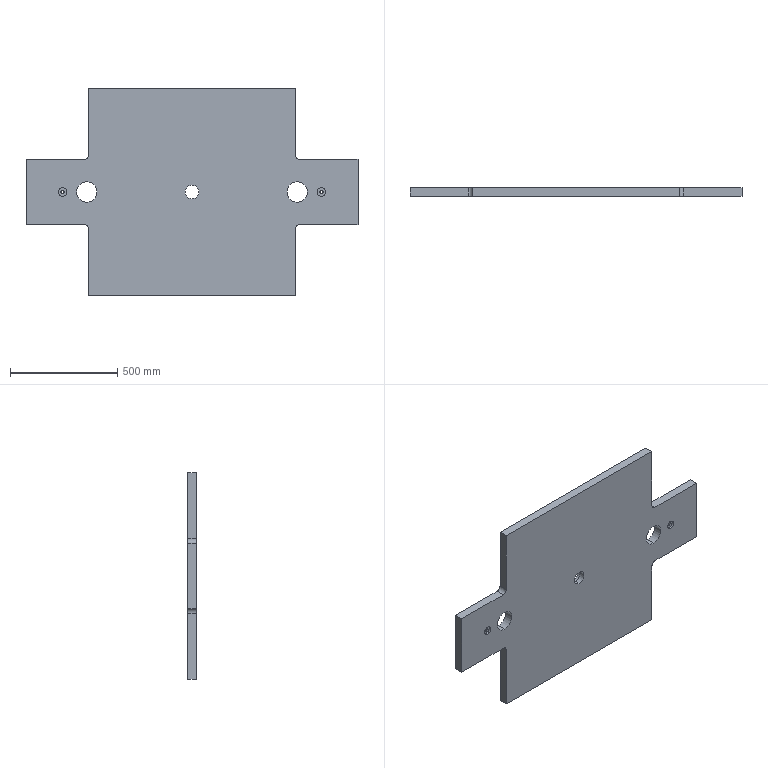Part | SolidWorks | features Cut 4, MirrorPattern 2, Extrusion 1, Fillet 1, HoleWzd 1 | 1 solid | 43 faces | box 1546 x 40 x 960 mm | volume 43281864 mm3 | cylinder 24 | plane 19 | commonest cylinder face diameters 40 x8 15.5 x4 24 x4 95 x4 63.5 x2 68 x2
STEP:
#1=CARTESIAN_POINT('',(0.,25.,-34.));
#2=VERTEX_POINT('',#1);
#3=CARTESIAN_POINT('',(0.,25.,34.));
#4=VERTEX_POINT('',#3);
#5=CARTESIAN_POINT('',(0.,25.,0.));
#6=DIRECTION('',(0.,1.,0.));
#7=DIRECTION('',(0.,0.,1.));
#8=AXIS2_PLACEMENT_3D('',#5,#6,#7);
#9=CIRCLE('',#8,34.);
#10=EDGE_CURVE('',#2,#4,#9,.T.);
#11=ORIENTED_EDGE('',*,*,#10,.F.);
#12=CARTESIAN_POINT('',(0.,40.,-34.));
#13=VERTEX_POINT('',#12);
#14=CARTESIAN_POINT('',(0.,25.,-34.));
#15=DIRECTION('',(0.,1.,0.));
#16=VECTOR('',#15,1000.);
#17=LINE('',#14,#16);
#18=EDGE_CURVE('',#2,#13,#17,.T.);
#19=ORIENTED_EDGE('',*,*,#18,.T.);
#20=CARTESIAN_POINT('',(0.,40.,34.));
#21=VERTEX_POINT('',#20);
#22=CARTESIAN_POINT('',(0.,40.,0.));
#23=DIRECTION('',(0.,1.,0.));
#24=DIRECTION('',(0.,0.,1.));
#25=AXIS2_PLACEMENT_3D('',#22,#23,#24);
#26=CIRCLE('',#25,34.);
#27=EDGE_CURVE('',#13,#21,#26,.T.);
#28=ORIENTED_EDGE('',*,*,#27,.T.);
#29=CARTESIAN_POINT('',(0.,25.,34.));
#30=DIRECTION('',(0.,1.,0.));
#31=VECTOR('',#30,1000.);
#32=LINE('',#29,#31);
#33=EDGE_CURVE('',#4,#21,#32,.T.);
#34=ORIENTED_EDGE('',*,*,#33,.F.);
#35=EDGE_LOOP('',(#11,#19,#28,#34));
#36=FACE_OUTER_BOUND('',#35,.T.);
#37=CARTESIAN_POINT('',(0.,25.,0.));
#38=DIRECTION('',(0.,1.,0.));
#39=DIRECTION('',(0.,0.,1.));
#40=AXIS2_PLACEMENT_3D('',#37,#38,#39);
#41=CYLINDRICAL_SURFACE('',#40,34.);
#42=ADVANCED_FACE('',(#36),#41,.F.);
#43=CARTESIAN_POINT('',(-490.,40.,-47.5));
#44=VERTEX_POINT('',#43);
#45=CARTESIAN_POINT('',(-490.,40.,47.5));
#46=VERTEX_POINT('',#45);
#47=CARTESIAN_POINT('',(-490.,40.,0.));
#48=DIRECTION('',(0.,1.,0.));
#49=DIRECTION('',(0.,0.,-1.));
#50=AXIS2_PLACEMENT_3D('',#47,#48,#49);
#51=CIRCLE('',#50,47.5);
#52=EDGE_CURVE('',#44,#46,#51,.T.);
#53=ORIENTED_EDGE('',*,*,#52,.T.);
#54=CARTESIAN_POINT('',(-490.,0.,47.5));
#55=VERTEX_POINT('',#54);
#56=CARTESIAN_POINT('',(-490.,40.,47.5));
#57=DIRECTION('',(0.,-1.,0.));
#58=VECTOR('',#57,1000.);
#59=LINE('',#56,#58);
#60=EDGE_CURVE('',#46,#55,#59,.T.);
#61=ORIENTED_EDGE('',*,*,#60,.T.);
#62=CARTESIAN_POINT('',(-490.,0.,-47.5));
#63=VERTEX_POINT('',#62);
#64=CARTESIAN_POINT('',(-490.,0.,0.));
#65=DIRECTION('',(0.,1.,0.));
#66=DIRECTION('',(0.,0.,-1.));
#67=AXIS2_PLACEMENT_3D('',#64,#65,#66);
#68=CIRCLE('',#67,47.5);
#69=EDGE_CURVE('',#63,#55,#68,.T.);
#70=ORIENTED_EDGE('',*,*,#69,.F.);
#71=CARTESIAN_POINT('',(-490.,40.,-47.5));
#72=DIRECTION('',(0.,-1.,0.));
#73=VECTOR('',#72,1000.);
#74=LINE('',#71,#73);
#75=EDGE_CURVE('',#44,#63,#74,.T.);
#76=ORIENTED_EDGE('',*,*,#75,.F.);
#77=EDGE_LOOP('',(#53,#61,#70,#76));
#78=FACE_OUTER_BOUND('',#77,.T.);
#79=CARTESIAN_POINT('',(-490.,40.,0.));
#80=DIRECTION('',(0.,-1.,0.));
#81=DIRECTION('',(0.,0.,-1.));
#82=AXIS2_PLACEMENT_3D('',#79,#80,#81);
#83=CYLINDRICAL_SURFACE('',#82,47.5);
#84=ADVANCED_FACE('',(#78),#83,.F.);
#85=CARTESIAN_POINT('',(490.,40.,47.5));
#86=VERTEX_POINT('',#85);
#87=CARTESIAN_POINT('',(490.,40.,-47.5));
#88=VERTEX_POINT('',#87);
#89=CARTESIAN_POINT('',(490.,40.,0.));
#90=DIRECTION('',(0.,-1.,0.));
#91=DIRECTION('',(0.,0.,-1.));
#92=AXIS2_PLACEMENT_3D('',#89,#90,#91);
#93=CIRCLE('',#92,47.5);
#94=EDGE_CURVE('',#86,#88,#93,.T.);
#95=ORIENTED_EDGE('',*,*,#94,.F.);
#96=CARTESIAN_POINT('',(490.,0.,47.5));
#97=VERTEX_POINT('',#96);
#98=CARTESIAN_POINT('',(490.,40.,47.5));
#99=DIRECTION('',(0.,-1.,0.));
#100=VECTOR('',#99,1000.);
#101=LINE('',#98,#100);
#102=EDGE_CURVE('',#86,#97,#101,.T.);
#103=ORIENTED_EDGE('',*,*,#102,.T.);
#104=CARTESIAN_POINT('',(490.,0.,-47.5));
#105=VERTEX_POINT('',#104);
#106=CARTESIAN_POINT('',(490.,0.,0.));
#107=DIRECTION('',(0.,-1.,0.));
#108=DIRECTION('',(0.,0.,-1.));
#109=AXIS2_PLACEMENT_3D('',#106,#107,#108);
#110=CIRCLE('',#109,47.5);
#111=EDGE_CURVE('',#97,#105,#110,.T.);
#112=ORIENTED_EDGE('',*,*,#111,.T.);
#113=CARTESIAN_POINT('',(490.,40.,-47.5));
#114=DIRECTION('',(0.,-1.,0.));
#115=VECTOR('',#114,1000.);
#116=LINE('',#113,#115);
#117=EDGE_CURVE('',#88,#105,#116,.T.);
#118=ORIENTED_EDGE('',*,*,#117,.F.);
#119=EDGE_LOOP('',(#95,#103,#112,#118));
#120=FACE_OUTER_BOUND('',#119,.T.);
#121=CARTESIAN_POINT('',(490.,40.,0.));
#122=DIRECTION('',(0.,-1.,0.));
#123=DIRECTION('',(0.,0.,-1.));
#124=AXIS2_PLACEMENT_3D('',#121,#122,#123);
#125=CYLINDRICAL_SURFACE('',#124,47.5);
#126=ADVANCED_FACE('',(#120),#125,.F.);
#127=CARTESIAN_POINT('',(-602.5,25.,-12.));
#128=VERTEX_POINT('',#127);
#129=CARTESIAN_POINT('',(-602.5,25.,12.));
#130=VERTEX_POINT('',#129);
#131=CARTESIAN_POINT('',(-602.5,25.,0.));
#132=DIRECTION('',(0.,1.,0.));
#133=DIRECTION('',(0.,0.,1.));
#134=AXIS2_PLACEMENT_3D('',#131,#132,#133);
#135=CIRCLE('',#134,12.);
#136=EDGE_CURVE('',#128,#130,#135,.T.);
#137=ORIENTED_EDGE('',*,*,#136,.F.);
#138=CARTESIAN_POINT('',(-602.5,40.,-12.));
#139=VERTEX_POINT('',#138);
#140=CARTESIAN_POINT('',(-602.5,40.,-12.));
#141=DIRECTION('',(0.,1.,0.));
#142=VECTOR('',#141,1000.);
#143=LINE('',#140,#142);
#144=EDGE_CURVE('',#128,#139,#143,.T.);
#145=ORIENTED_EDGE('',*,*,#144,.T.);
#146=CARTESIAN_POINT('',(-602.5,40.,12.));
#147=VERTEX_POINT('',#146);
#148=CARTESIAN_POINT('',(-602.5,40.,0.));
#149=DIRECTION('',(0.,1.,0.));
#150=DIRECTION('',(0.,0.,1.));
#151=AXIS2_PLACEMENT_3D('',#148,#149,#150);
#152=CIRCLE('',#151,12.);
#153=EDGE_CURVE('',#139,#147,#152,.T.);
#154=ORIENTED_EDGE('',*,*,#153,.T.);
#155=CARTESIAN_POINT('',(-602.5,40.,12.));
#156=DIRECTION('',(0.,1.,0.));
#157=VECTOR('',#156,1000.);
#158=LINE('',#155,#157);
#159=EDGE_CURVE('',#130,#147,#158,.T.);
#160=ORIENTED_EDGE('',*,*,#159,.F.);
#161=EDGE_LOOP('',(#137,#145,#154,#160));
#162=FACE_OUTER_BOUND('',#161,.T.);
#163=CARTESIAN_POINT('',(-602.5,40.,0.));
#164=DIRECTION('',(0.,1.,0.));
#165=DIRECTION('',(0.,0.,1.));
#166=AXIS2_PLACEMENT_3D('',#163,#164,#165);
#167=CYLINDRICAL_SURFACE('',#166,12.);
#168=ADVANCED_FACE('',(#162),#167,.F.);
#169=CARTESIAN_POINT('',(-602.5,10.,7.75));
#170=VERTEX_POINT('',#169);
#171=CARTESIAN_POINT('',(-602.5,10.,-7.75));
#172=VERTEX_POINT('',#171);
#173=CARTESIAN_POINT('',(-602.5,10.,0.));
#174=DIRECTION('',(0.,-1.,0.));
#175=DIRECTION('',(0.,0.,-1.));
#176=AXIS2_PLACEMENT_3D('',#173,#174,#175);
#177=CIRCLE('',#176,7.75);
#178=EDGE_CURVE('',#170,#172,#177,.T.);
#179=ORIENTED_EDGE('',*,*,#178,.T.);
#180=CARTESIAN_POINT('',(-602.5,25.,-7.75));
#181=VERTEX_POINT('',#180);
#182=CARTESIAN_POINT('',(-602.5,40.,-7.75));
#183=DIRECTION('',(0.,1.,0.));
#184=VECTOR('',#183,1000.);
#185=LINE('',#182,#184);
#186=EDGE_CURVE('',#172,#181,#185,.T.);
#187=ORIENTED_EDGE('',*,*,#186,.T.);
#188=CARTESIAN_POINT('',(-602.5,25.,7.75));
#189=VERTEX_POINT('',#188);
#190=CARTESIAN_POINT('',(-602.5,25.,0.));
#191=DIRECTION('',(0.,1.,0.));
#192=DIRECTION('',(0.,0.,1.));
#193=AXIS2_PLACEMENT_3D('',#190,#191,#192);
#194=CIRCLE('',#193,7.75);
#195=EDGE_CURVE('',#181,#189,#194,.T.);
#196=ORIENTED_EDGE('',*,*,#195,.T.);
#197=CARTESIAN_POINT('',(-602.5,40.,7.75));
#198=DIRECTION('',(0.,1.,0.));
#199=VECTOR('',#198,1000.);
#200=LINE('',#197,#199);
#201=EDGE_CURVE('',#170,#189,#200,.T.);
#202=ORIENTED_EDGE('',*,*,#201,.F.);
#203=EDGE_LOOP('',(#179,#187,#196,#202));
#204=FACE_OUTER_BOUND('',#203,.T.);
#205=CARTESIAN_POINT('',(-602.5,40.,0.));
#206=DIRECTION('',(0.,1.,0.));
#207=DIRECTION('',(0.,0.,1.));
#208=AXIS2_PLACEMENT_3D('',#205,#206,#207);
#209=CYLINDRICAL_SURFACE('',#208,7.75);
#210=ADVANCED_FACE('',(#204),#209,.F.);
#211=CARTESIAN_POINT('',(-602.5,10.,-20.));
#212=VERTEX_POINT('',#211);
#213=CARTESIAN_POINT('',(-602.5,10.,20.));
#214=VERTEX_POINT('',#213);
#215=CARTESIAN_POINT('',(-602.5,10.,0.));
#216=DIRECTION('',(0.,1.,0.));
#217=DIRECTION('',(0.,0.,-1.));
#218=AXIS2_PLACEMENT_3D('',#215,#216,#217);
#219=CIRCLE('',#218,20.);
#220=EDGE_CURVE('',#212,#214,#219,.T.);
#221=ORIENTED_EDGE('',*,*,#220,.T.);
#222=CARTESIAN_POINT('',(-602.5,0.,20.));
#223=VERTEX_POINT('',#222);
#224=CARTESIAN_POINT('',(-602.5,10.,20.));
#225=DIRECTION('',(0.,-1.,0.));
#226=VECTOR('',#225,1000.);
#227=LINE('',#224,#226);
#228=EDGE_CURVE('',#214,#223,#227,.T.);
#229=ORIENTED_EDGE('',*,*,#228,.T.);
#230=CARTESIAN_POINT('',(-602.5,0.,-20.));
#231=VERTEX_POINT('',#230);
#232=CARTESIAN_POINT('',(-602.5,0.,0.));
#233=DIRECTION('',(0.,1.,0.));
#234=DIRECTION('',(0.,0.,-1.));
#235=AXIS2_PLACEMENT_3D('',#232,#233,#234);
#236=CIRCLE('',#235,20.);
#237=EDGE_CURVE('',#231,#223,#236,.T.);
#238=ORIENTED_EDGE('',*,*,#237,.F.);
#239=CARTESIAN_POINT('',(-602.5,10.,-20.));
#240=DIRECTION('',(0.,-1.,0.));
#241=VECTOR('',#240,1000.);
#242=LINE('',#239,#241);
#243=EDGE_CURVE('',#212,#231,#242,.T.);
#244=ORIENTED_EDGE('',*,*,#243,.F.);
#245=EDGE_LOOP('',(#221,#229,#238,#244));
#246=FACE_OUTER_BOUND('',#245,.T.);
#247=CARTESIAN_POINT('',(-602.5,10.,0.));
#248=DIRECTION('',(0.,-1.,0.));
#249=DIRECTION('',(0.,0.,-1.));
#250=AXIS2_PLACEMENT_3D('',#247,#248,#249);
#251=CYLINDRICAL_SURFACE('',#250,20.);
#252=ADVANCED_FACE('',(#246),#251,.F.);
#253=CARTESIAN_POINT('',(602.5,25.,-12.));
#254=VERTEX_POINT('',#253);
#255=CARTESIAN_POINT('',(602.5,25.,12.));
#256=VERTEX_POINT('',#255);
#257=CARTESIAN_POINT('',(602.5,25.,0.));
#258=DIRECTION('',(0.,1.,0.));
#259=DIRECTION('',(0.,0.,1.));
#260=AXIS2_PLACEMENT_3D('',#257,#258,#259);
#261=CIRCLE('',#260,12.);
#262=EDGE_CURVE('',#254,#256,#261,.T.);
#263=ORIENTED_EDGE('',*,*,#262,.F.);
#264=CARTESIAN_POINT('',(602.5,40.,-12.));
#265=VERTEX_POINT('',#264);
#266=CARTESIAN_POINT('',(602.5,40.,-12.));
#267=DIRECTION('',(0.,1.,0.));
#268=VECTOR('',#267,1000.);
#269=LINE('',#266,#268);
#270=EDGE_CURVE('',#254,#265,#269,.T.);
#271=ORIENTED_EDGE('',*,*,#270,.T.);
#272=CARTESIAN_POINT('',(602.5,40.,12.));
#273=VERTEX_POINT('',#272);
#274=CARTESIAN_POINT('',(602.5,40.,0.));
#275=DIRECTION('',(0.,1.,0.));
#276=DIRECTION('',(0.,0.,1.));
#277=AXIS2_PLACEMENT_3D('',#274,#275,#276);
#278=CIRCLE('',#277,12.);
#279=EDGE_CURVE('',#265,#273,#278,.T.);
#280=ORIENTED_EDGE('',*,*,#279,.T.);
#281=CARTESIAN_POINT('',(602.5,40.,12.));
#282=DIRECTION('',(0.,1.,0.));
#283=VECTOR('',#282,1000.);
#284=LINE('',#281,#283);
#285=EDGE_CURVE('',#256,#273,#284,.T.);
#286=ORIENTED_EDGE('',*,*,#285,.F.);
#287=EDGE_LOOP('',(#263,#271,#280,#286));
#288=FACE_OUTER_BOUND('',#287,.T.);
#289=CARTESIAN_POINT('',(602.5,40.,0.));
#290=DIRECTION('',(0.,1.,0.));
#291=DIRECTION('',(0.,0.,1.));
#292=AXIS2_PLACEMENT_3D('',#289,#290,#291);
#293=CYLINDRICAL_SURFACE('',#292,12.);
#294=ADVANCED_FACE('',(#288),#293,.F.);
#295=CARTESIAN_POINT('',(602.5,10.,7.75));
#296=VERTEX_POINT('',#295);
#297=CARTESIAN_POINT('',(602.5,10.,-7.75));
#298=VERTEX_POINT('',#297);
#299=CARTESIAN_POINT('',(602.5,10.,0.));
#300=DIRECTION('',(0.,-1.,0.));
#301=DIRECTION('',(0.,0.,-1.));
#302=AXIS2_PLACEMENT_3D('',#299,#300,#301);
#303=CIRCLE('',#302,7.75);
#304=EDGE_CURVE('',#296,#298,#303,.T.);
#305=ORIENTED_EDGE('',*,*,#304,.T.);
#306=CARTESIAN_POINT('',(602.5,25.,-7.75));
#307=VERTEX_POINT('',#306);
#308=CARTESIAN_POINT('',(602.5,40.,-7.75));
#309=DIRECTION('',(0.,1.,0.));
#310=VECTOR('',#309,1000.);
#311=LINE('',#308,#310);
#312=EDGE_CURVE('',#298,#307,#311,.T.);
#313=ORIENTED_EDGE('',*,*,#312,.T.);
#314=CARTESIAN_POINT('',(602.5,25.,7.75));
#315=VERTEX_POINT('',#314);
#316=CARTESIAN_POINT('',(602.5,25.,0.));
#317=DIRECTION('',(0.,1.,0.));
#318=DIRECTION('',(0.,0.,1.));
#319=AXIS2_PLACEMENT_3D('',#316,#317,#318);
#320=CIRCLE('',#319,7.75);
#321=EDGE_CURVE('',#307,#315,#320,.T.);
#322=ORIENTED_EDGE('',*,*,#321,.T.);
#323=CARTESIAN_POINT('',(602.5,40.,7.75));
#324=DIRECTION('',(0.,1.,0.));
#325=VECTOR('',#324,1000.);
#326=LINE('',#323,#325);
#327=EDGE_CURVE('',#296,#315,#326,.T.);
#328=ORIENTED_EDGE('',*,*,#327,.F.);
#329=EDGE_LOOP('',(#305,#313,#322,#328));
#330=FACE_OUTER_BOUND('',#329,.T.);
#331=CARTESIAN_POINT('',(602.5,40.,0.));
#332=DIRECTION('',(0.,1.,0.));
#333=DIRECTION('',(0.,0.,1.));
#334=AXIS2_PLACEMENT_3D('',#331,#332,#333);
#335=CYLINDRICAL_SURFACE('',#334,7.75);
#336=ADVANCED_FACE('',(#330),#335,.F.);
#337=CARTESIAN_POINT('',(602.5,10.,20.));
#338=VERTEX_POINT('',#337);
#339=CARTESIAN_POINT('',(602.5,10.,-20.));
#340=VERTEX_POINT('',#339);
#341=CARTESIAN_POINT('',(602.5,10.,0.));
#342=DIRECTION('',(0.,-1.,0.));
#343=DIRECTION('',(0.,0.,-1.));
#344=AXIS2_PLACEMENT_3D('',#341,#342,#343);
#345=CIRCLE('',#344,20.);
#346=EDGE_CURVE('',#338,#340,#345,.T.);
#347=ORIENTED_EDGE('',*,*,#346,.F.);
#348=CARTESIAN_POINT('',(602.5,0.,20.));
#349=VERTEX_POINT('',#348);
#350=CARTESIAN_POINT('',(602.5,10.,20.));
#351=DIRECTION('',(0.,-1.,0.));
#352=VECTOR('',#351,1000.);
#353=LINE('',#350,#352);
#354=EDGE_CURVE('',#338,#349,#353,.T.);
#355=ORIENTED_EDGE('',*,*,#354,.T.);
#356=CARTESIAN_POINT('',(602.5,0.,-20.));
#357=VERTEX_POINT('',#356);
#358=CARTESIAN_POINT('',(602.5,0.,0.));
#359=DIRECTION('',(0.,-1.,0.));
#360=DIRECTION('',(0.,0.,-1.));
#361=AXIS2_PLACEMENT_3D('',#358,#359,#360);
#362=CIRCLE('',#361,20.);
#363=EDGE_CURVE('',#349,#357,#362,.T.);
#364=ORIENTED_EDGE('',*,*,#363,.T.);
#365=CARTESIAN_POINT('',(602.5,10.,-20.));
#366=DIRECTION('',(0.,-1.,0.));
#367=VECTOR('',#366,1000.);
#368=LINE('',#365,#367);
#369=EDGE_CURVE('',#340,#357,#368,.T.);
#370=ORIENTED_EDGE('',*,*,#369,.F.);
#371=EDGE_LOOP('',(#347,#355,#364,#370));
#372=FACE_OUTER_BOUND('',#371,.T.);
#373=CARTESIAN_POINT('',(602.5,10.,0.));
#374=DIRECTION('',(0.,-1.,0.));
#375=DIRECTION('',(0.,0.,-1.));
#376=AXIS2_PLACEMENT_3D('',#373,#374,#375);
#377=CYLINDRICAL_SURFACE('',#376,20.);
#378=ADVANCED_FACE('',(#372),#377,.F.);
#379=CARTESIAN_POINT('',(0.,0.,-31.75));
#380=VERTEX_POINT('',#379);
#381=CARTESIAN_POINT('',(0.,0.,31.75));
#382=VERTEX_POINT('',#381);
#383=CARTESIAN_POINT('',(0.,0.,0.));
#384=DIRECTION('',(0.,1.,0.));
#385=DIRECTION('',(0.,0.,1.));
#386=AXIS2_PLACEMENT_3D('',#383,#384,#385);
#387=CIRCLE('',#386,31.75);
#388=EDGE_CURVE('',#380,#382,#387,.T.);
#389=ORIENTED_EDGE('',*,*,#388,.F.);
#390=CARTESIAN_POINT('',(0.,25.,-31.75));
#391=VERTEX_POINT('',#390);
#392=CARTESIAN_POINT('',(0.,0.,-31.75));
#393=DIRECTION('',(0.,1.,0.));
#394=VECTOR('',#393,1000.);
#395=LINE('',#392,#394);
#396=EDGE_CURVE('',#380,#391,#395,.T.);
#397=ORIENTED_EDGE('',*,*,#396,.T.);
#398=CARTESIAN_POINT('',(0.,25.,31.75));
#399=VERTEX_POINT('',#398);
#400=CARTESIAN_POINT('',(0.,25.,0.));
#401=DIRECTION('',(0.,-1.,0.));
#402=DIRECTION('',(0.,0.,1.));
#403=AXIS2_PLACEMENT_3D('',#400,#401,#402);
#404=CIRCLE('',#403,31.75);
#405=EDGE_CURVE('',#399,#391,#404,.T.);
#406=ORIENTED_EDGE('',*,*,#405,.F.);
#407=CARTESIAN_POINT('',(0.,0.,31.75));
#408=DIRECTION('',(0.,1.,0.));
#409=VECTOR('',#408,1000.);
#410=LINE('',#407,#409);
#411=EDGE_CURVE('',#382,#399,#410,.T.);
#412=ORIENTED_EDGE('',*,*,#411,.F.);
#413=EDGE_LOOP('',(#389,#397,#406,#412));
#414=FACE_OUTER_BOUND('',#413,.T.);
#415=CARTESIAN_POINT('',(0.,0.,0.));
#416=DIRECTION('',(0.,1.,0.));
#417=DIRECTION('',(0.,0.,1.));
#418=AXIS2_PLACEMENT_3D('',#415,#416,#417);
#419=CYLINDRICAL_SURFACE('',#418,31.75);
#420=ADVANCED_FACE('',(#414),#419,.F.);
#421=ORIENTED_EDGE('',*,*,#396,.F.);
#422=CARTESIAN_POINT('',(0.,0.,0.));
#423=DIRECTION('',(0.,1.,0.));
#424=DIRECTION('',(0.,0.,1.));
#425=AXIS2_PLACEMENT_3D('',#422,#423,#424);
#426=CIRCLE('',#425,31.75);
#427=EDGE_CURVE('',#382,#380,#426,.T.);
#428=ORIENTED_EDGE('',*,*,#427,.F.);
#429=ORIENTED_EDGE('',*,*,#411,.T.);
#430=CARTESIAN_POINT('',(0.,25.,0.));
#431=DIRECTION('',(0.,-1.,0.));
#432=DIRECTION('',(0.,0.,1.));
#433=AXIS2_PLACEMENT_3D('',#430,#431,#432);
#434=CIRCLE('',#433,31.75);
#435=EDGE_CURVE('',#391,#399,#434,.T.);
#436=ORIENTED_EDGE('',*,*,#435,.F.);
#437=EDGE_LOOP('',(#421,#428,#429,#436));
#438=FACE_OUTER_BOUND('',#437,.T.);
#439=CARTESIAN_POINT('',(0.,0.,0.));
#440=DIRECTION('',(0.,1.,0.));
#441=DIRECTION('',(0.,0.,1.));
#442=AXIS2_PLACEMENT_3D('',#439,#440,#441);
#443=CYLINDRICAL_SURFACE('',#442,31.75);
#444=ADVANCED_FACE('',(#438),#443,.F.);
#445=CARTESIAN_POINT('',(-480.,40.,172.5));
#446=VERTEX_POINT('',#445);
#447=CARTESIAN_POINT('',(-480.,40.,480.));
#448=VERTEX_POINT('',#447);
#449=CARTESIAN_POINT('',(-480.,40.,480.));
#450=DIRECTION('',(0.,0.,1.));
#451=VECTOR('',#450,1000.);
#452=LINE('',#449,#451);
#453=EDGE_CURVE('',#446,#448,#452,.T.);
#454=ORIENTED_EDGE('',*,*,#453,.F.);
#455=CARTESIAN_POINT('',(-480.,0.,172.5));
#456=VERTEX_POINT('',#455);
#457=CARTESIAN_POINT('',(-480.,0.,172.5));
#458=DIRECTION('',(0.,-1.,0.));
#459=VECTOR('',#458,1000.);
#460=LINE('',#457,#459);
#461=EDGE_CURVE('',#446,#456,#460,.T.);
#462=ORIENTED_EDGE('',*,*,#461,.T.);
#463=CARTESIAN_POINT('',(-480.,0.,480.));
#464=VERTEX_POINT('',#463);
#465=CARTESIAN_POINT('',(-480.,0.,480.));
#466=DIRECTION('',(0.,0.,1.));
#467=VECTOR('',#466,1000.);
#468=LINE('',#465,#467);
#469=EDGE_CURVE('',#456,#464,#468,.T.);
#470=ORIENTED_EDGE('',*,*,#469,.T.);
#471=CARTESIAN_POINT('',(-480.,40.,480.));
#472=DIRECTION('',(0.,-1.,0.));
#473=VECTOR('',#472,1000.);
#474=LINE('',#471,#473);
#475=EDGE_CURVE('',#448,#464,#474,.T.);
#476=ORIENTED_EDGE('',*,*,#475,.F.);
#477=EDGE_LOOP('',(#454,#462,#470,#476));
#478=FACE_OUTER_BOUND('',#477,.T.);
#479=CARTESIAN_POINT('',(-480.,40.,480.));
#480=DIRECTION('',(1.,0.,0.));
#481=DIRECTION('',(0.,0.,-1.));
#482=AXIS2_PLACEMENT_3D('',#479,#480,#481);
#483=PLANE('',#482);
#484=ADVANCED_FACE('',(#478),#483,.F.);
#485=CARTESIAN_POINT('',(480.,0.,480.));
#486=VERTEX_POINT('',#485);
#487=CARTESIAN_POINT('',(480.,0.,480.));
#488=DIRECTION('',(1.,0.,0.));
#489=VECTOR('',#488,1000.);
#490=LINE('',#487,#489);
#491=EDGE_CURVE('',#464,#486,#490,.T.);
#492=ORIENTED_EDGE('',*,*,#491,.T.);
#493=CARTESIAN_POINT('',(480.,40.,480.));
#494=VERTEX_POINT('',#493);
#495=CARTESIAN_POINT('',(480.,40.,480.));
#496=DIRECTION('',(0.,-1.,0.));
#497=VECTOR('',#496,1000.);
#498=LINE('',#495,#497);
#499=EDGE_CURVE('',#494,#486,#498,.T.);
#500=ORIENTED_EDGE('',*,*,#499,.F.);
#501=CARTESIAN_POINT('',(480.,40.,480.));
#502=DIRECTION('',(1.,0.,0.));
#503=VECTOR('',#502,1000.);
#504=LINE('',#501,#503);
#505=EDGE_CURVE('',#448,#494,#504,.T.);
#506=ORIENTED_EDGE('',*,*,#505,.F.);
#507=ORIENTED_EDGE('',*,*,#475,.T.);
#508=EDGE_LOOP('',(#492,#500,#506,#507));
#509=FACE_OUTER_BOUND('',#508,.T.);
#510=CARTESIAN_POINT('',(480.,40.,480.));
#511=DIRECTION('',(0.,0.,-1.));
#512=DIRECTION('',(-1.,0.,0.));
#513=AXIS2_PLACEMENT_3D('',#510,#511,#512);
#514=PLANE('',#513);
#515=ADVANCED_FACE('',(#509),#514,.F.);
#516=CARTESIAN_POINT('',(480.,0.,172.5));
#517=VERTEX_POINT('',#516);
#518=CARTESIAN_POINT('',(480.,0.,152.5));
#519=DIRECTION('',(0.,0.,-1.));
#520=VECTOR('',#519,1000.);
#521=LINE('',#518,#520);
#522=EDGE_CURVE('',#486,#517,#521,.T.);
#523=ORIENTED_EDGE('',*,*,#522,.T.);
#524=CARTESIAN_POINT('',(480.,40.,172.5));
#525=VERTEX_POINT('',#524);
#526=CARTESIAN_POINT('',(480.,40.,172.5));
#527=DIRECTION('',(0.,1.,0.));
#528=VECTOR('',#527,1000.);
#529=LINE('',#526,#528);
#530=EDGE_CURVE('',#517,#525,#529,.T.);
#531=ORIENTED_EDGE('',*,*,#530,.T.);
#532=CARTESIAN_POINT('',(480.,40.,152.5));
#533=DIRECTION('',(0.,0.,-1.));
#534=VECTOR('',#533,1000.);
#535=LINE('',#532,#534);
#536=EDGE_CURVE('',#494,#525,#535,.T.);
#537=ORIENTED_EDGE('',*,*,#536,.F.);
#538=ORIENTED_EDGE('',*,*,#499,.T.);
#539=EDGE_LOOP('',(#523,#531,#537,#538));
#540=FACE_OUTER_BOUND('',#539,.T.);
#541=CARTESIAN_POINT('',(480.,40.,152.5));
#542=DIRECTION('',(-1.,0.,0.));
#543=DIRECTION('',(0.,0.,1.));
#544=AXIS2_PLACEMENT_3D('',#541,#542,#543);
#545=PLANE('',#544);
#546=ADVANCED_FACE('',(#540),#545,.F.);
#547=CARTESIAN_POINT('',(500.,40.,152.5));
#548=VERTEX_POINT('',#547);
#549=CARTESIAN_POINT('',(773.,40.,152.5));
#550=VERTEX_POINT('',#549);
#551=CARTESIAN_POINT('',(773.,40.,152.5));
#552=DIRECTION('',(1.,0.,0.));
#553=VECTOR('',#552,1000.);
#554=LINE('',#551,#553);
#555=EDGE_CURVE('',#548,#550,#554,.T.);
#556=ORIENTED_EDGE('',*,*,#555,.F.);
#557=CARTESIAN_POINT('',(500.,0.,152.5));
#558=VERTEX_POINT('',#557);
#559=CARTESIAN_POINT('',(500.,0.,152.5));
#560=DIRECTION('',(0.,-1.,0.));
#561=VECTOR('',#560,1000.);
#562=LINE('',#559,#561);
#563=EDGE_CURVE('',#548,#558,#562,.T.);
#564=ORIENTED_EDGE('',*,*,#563,.T.);
#565=CARTESIAN_POINT('',(773.,0.,152.5));
#566=VERTEX_POINT('',#565);
#567=CARTESIAN_POINT('',(773.,0.,152.5));
#568=DIRECTION('',(1.,0.,0.));
#569=VECTOR('',#568,1000.);
#570=LINE('',#567,#569);
#571=EDGE_CURVE('',#558,#566,#570,.T.);
#572=ORIENTED_EDGE('',*,*,#571,.T.);
#573=CARTESIAN_POINT('',(773.,40.,152.5));
#574=DIRECTION('',(0.,-1.,0.));
#575=VECTOR('',#574,1000.);
#576=LINE('',#573,#575);
#577=EDGE_CURVE('',#550,#566,#576,.T.);
#578=ORIENTED_EDGE('',*,*,#577,.F.);
#579=EDGE_LOOP('',(#556,#564,#572,#578));
#580=FACE_OUTER_BOUND('',#579,.T.);
#581=CARTESIAN_POINT('',(773.,40.,152.5));
#582=DIRECTION('',(0.,0.,-1.));
#583=DIRECTION('',(-1.,0.,0.));
#584=AXIS2_PLACEMENT_3D('',#581,#582,#583);
#585=PLANE('',#584);
#586=ADVANCED_FACE('',(#580),#585,.F.);
#587=CARTESIAN_POINT('',(773.,0.,-152.5));
#588=VERTEX_POINT('',#587);
#589=CARTESIAN_POINT('',(773.,0.,-152.5));
#590=DIRECTION('',(0.,0.,-1.));
#591=VECTOR('',#590,1000.);
#592=LINE('',#589,#591);
#593=EDGE_CURVE('',#566,#588,#592,.T.);
#594=ORIENTED_EDGE('',*,*,#593,.T.);
#595=CARTESIAN_POINT('',(773.,40.,-152.5));
#596=VERTEX_POINT('',#595);
#597=CARTESIAN_POINT('',(773.,40.,-152.5));
#598=DIRECTION('',(0.,-1.,0.));
#599=VECTOR('',#598,1000.);
#600=LINE('',#597,#599);
#601=EDGE_CURVE('',#596,#588,#600,.T.);
#602=ORIENTED_EDGE('',*,*,#601,.F.);
#603=CARTESIAN_POINT('',(773.,40.,-152.5));
#604=DIRECTION('',(0.,0.,-1.));
#605=VECTOR('',#604,1000.);
#606=LINE('',#603,#605);
#607=EDGE_CURVE('',#550,#596,#606,.T.);
#608=ORIENTED_EDGE('',*,*,#607,.F.);
#609=ORIENTED_EDGE('',*,*,#577,.T.);
#610=EDGE_LOOP('',(#594,#602,#608,#609));
#611=FACE_OUTER_BOUND('',#610,.T.);
#612=CARTESIAN_POINT('',(773.,40.,-152.5));
#613=DIRECTION('',(-1.,0.,0.));
#614=DIRECTION('',(0.,0.,1.));
#615=AXIS2_PLACEMENT_3D('',#612,#613,#614);
#616=PLANE('',#615);
#617=ADVANCED_FACE('',(#611),#616,.F.);
#618=CARTESIAN_POINT('',(500.,0.,-152.5));
#619=VERTEX_POINT('',#618);
#620=CARTESIAN_POINT('',(480.,0.,-152.5));
#621=DIRECTION('',(-1.,0.,0.));
#622=VECTOR('',#621,1000.);
#623=LINE('',#620,#622);
#624=EDGE_CURVE('',#588,#619,#623,.T.);
#625=ORIENTED_EDGE('',*,*,#624,.T.);
#626=CARTESIAN_POINT('',(500.,40.,-152.5));
#627=VERTEX_POINT('',#626);
#628=CARTESIAN_POINT('',(500.,40.,-152.5));
#629=DIRECTION('',(0.,1.,0.));
#630=VECTOR('',#629,1000.);
#631=LINE('',#628,#630);
#632=EDGE_CURVE('',#619,#627,#631,.T.);
#633=ORIENTED_EDGE('',*,*,#632,.T.);
#634=CARTESIAN_POINT('',(480.,40.,-152.5));
#635=DIRECTION('',(-1.,0.,0.));
#636=VECTOR('',#635,1000.);
#637=LINE('',#634,#636);
#638=EDGE_CURVE('',#596,#627,#637,.T.);
#639=ORIENTED_EDGE('',*,*,#638,.F.);
#640=ORIENTED_EDGE('',*,*,#601,.T.);
#641=EDGE_LOOP('',(#625,#633,#639,#640));
#642=FACE_OUTER_BOUND('',#641,.T.);
#643=CARTESIAN_POINT('',(480.,40.,-152.5));
#644=DIRECTION('',(0.,0.,1.));
#645=DIRECTION('',(1.,0.,0.));
#646=AXIS2_PLACEMENT_3D('',#643,#644,#645);
#647=PLANE('',#646);
#648=ADVANCED_FACE('',(#642),#647,.F.);
#649=CARTESIAN_POINT('',(480.,40.,-172.5));
#650=VERTEX_POINT('',#649);
#651=CARTESIAN_POINT('',(480.,40.,-480.));
#652=VERTEX_POINT('',#651);
#653=CARTESIAN_POINT('',(480.,40.,-480.));
#654=DIRECTION('',(0.,0.,-1.));
#655=VECTOR('',#654,1000.);
#656=LINE('',#653,#655);
#657=EDGE_CURVE('',#650,#652,#656,.T.);
#658=ORIENTED_EDGE('',*,*,#657,.F.);
#659=CARTESIAN_POINT('',(480.,0.,-172.5));
#660=VERTEX_POINT('',#659);
#661=CARTESIAN_POINT('',(480.,0.,-172.5));
#662=DIRECTION('',(0.,-1.,0.));
#663=VECTOR('',#662,1000.);
#664=LINE('',#661,#663);
#665=EDGE_CURVE('',#650,#660,#664,.T.);
#666=ORIENTED_EDGE('',*,*,#665,.T.);
#667=CARTESIAN_POINT('',(480.,0.,-480.));
#668=VERTEX_POINT('',#667);
#669=CARTESIAN_POINT('',(480.,0.,-480.));
#670=DIRECTION('',(0.,0.,-1.));
#671=VECTOR('',#670,1000.);
#672=LINE('',#669,#671);
#673=EDGE_CURVE('',#660,#668,#672,.T.);
#674=ORIENTED_EDGE('',*,*,#673,.T.);
#675=CARTESIAN_POINT('',(480.,40.,-480.));
#676=DIRECTION('',(0.,-1.,0.));
#677=VECTOR('',#676,1000.);
#678=LINE('',#675,#677);
#679=EDGE_CURVE('',#652,#668,#678,.T.);
#680=ORIENTED_EDGE('',*,*,#679,.F.);
#681=EDGE_LOOP('',(#658,#666,#674,#680));
#682=FACE_OUTER_BOUND('',#681,.T.);
#683=CARTESIAN_POINT('',(480.,40.,-480.));
#684=DIRECTION('',(-1.,0.,0.));
#685=DIRECTION('',(0.,0.,1.));
#686=AXIS2_PLACEMENT_3D('',#683,#684,#685);
#687=PLANE('',#686);
#688=ADVANCED_FACE('',(#682),#687,.F.);
#689=CARTESIAN_POINT('',(-480.,0.,-480.));
#690=VERTEX_POINT('',#689);
#691=CARTESIAN_POINT('',(-480.,0.,-480.));
#692=DIRECTION('',(-1.,0.,0.));
#693=VECTOR('',#692,1000.);
#694=LINE('',#691,#693);
#695=EDGE_CURVE('',#668,#690,#694,.T.);
#696=ORIENTED_EDGE('',*,*,#695,.T.);
#697=CARTESIAN_POINT('',(-480.,40.,-480.));
#698=VERTEX_POINT('',#697);
#699=CARTESIAN_POINT('',(-480.,40.,-480.));
#700=DIRECTION('',(0.,-1.,0.));
#701=VECTOR('',#700,1000.);
#702=LINE('',#699,#701);
#703=EDGE_CURVE('',#698,#690,#702,.T.);
#704=ORIENTED_EDGE('',*,*,#703,.F.);
#705=CARTESIAN_POINT('',(-480.,40.,-480.));
#706=DIRECTION('',(-1.,0.,0.));
#707=VECTOR('',#706,1000.);
#708=LINE('',#705,#707);
#709=EDGE_CURVE('',#652,#698,#708,.T.);
#710=ORIENTED_EDGE('',*,*,#709,.F.);
#711=ORIENTED_EDGE('',*,*,#679,.T.);
#712=EDGE_LOOP('',(#696,#704,#710,#711));
#713=FACE_OUTER_BOUND('',#712,.T.);
#714=CARTESIAN_POINT('',(-480.,40.,-480.));
#715=DIRECTION('',(0.,0.,1.));
#716=DIRECTION('',(1.,0.,0.));
#717=AXIS2_PLACEMENT_3D('',#714,#715,#716);
#718=PLANE('',#717);
#719=ADVANCED_FACE('',(#713),#718,.F.);
#720=CARTESIAN_POINT('',(-480.,0.,-172.5));
#721=VERTEX_POINT('',#720);
#722=CARTESIAN_POINT('',(-480.,0.,-152.5));
#723=DIRECTION('',(0.,0.,1.));
#724=VECTOR('',#723,1000.);
#725=LINE('',#722,#724);
#726=EDGE_CURVE('',#690,#721,#725,.T.);
#727=ORIENTED_EDGE('',*,*,#726,.T.);
#728=CARTESIAN_POINT('',(-480.,40.,-172.5));
#729=VERTEX_POINT('',#728);
#730=CARTESIAN_POINT('',(-480.,40.,-172.5));
#731=DIRECTION('',(0.,1.,0.));
#732=VECTOR('',#731,1000.);
#733=LINE('',#730,#732);
#734=EDGE_CURVE('',#721,#729,#733,.T.);
#735=ORIENTED_EDGE('',*,*,#734,.T.);
#736=CARTESIAN_POINT('',(-480.,40.,-152.5));
#737=DIRECTION('',(0.,0.,1.));
#738=VECTOR('',#737,1000.);
#739=LINE('',#736,#738);
#740=EDGE_CURVE('',#698,#729,#739,.T.);
#741=ORIENTED_EDGE('',*,*,#740,.F.);
#742=ORIENTED_EDGE('',*,*,#703,.T.);
#743=EDGE_LOOP('',(#727,#735,#741,#742));
#744=FACE_OUTER_BOUND('',#743,.T.);
#745=CARTESIAN_POINT('',(-480.,40.,-152.5));
#746=DIRECTION('',(1.,0.,0.));
#747=DIRECTION('',(0.,0.,-1.));
#748=AXIS2_PLACEMENT_3D('',#745,#746,#747);
#749=PLANE('',#748);
#750=ADVANCED_FACE('',(#744),#749,.F.);
#751=CARTESIAN_POINT('',(-500.,40.,-152.5));
#752=VERTEX_POINT('',#751);
#753=CARTESIAN_POINT('',(-773.,40.,-152.5));
#754=VERTEX_POINT('',#753);
#755=CARTESIAN_POINT('',(-773.,40.,-152.5));
#756=DIRECTION('',(-1.,0.,0.));
#757=VECTOR('',#756,1000.);
#758=LINE('',#755,#757);
#759=EDGE_CURVE('',#752,#754,#758,.T.);
#760=ORIENTED_EDGE('',*,*,#759,.F.);
#761=CARTESIAN_POINT('',(-500.,0.,-152.5));
#762=VERTEX_POINT('',#761);
#763=CARTESIAN_POINT('',(-500.,0.,-152.5));
#764=DIRECTION('',(0.,-1.,0.));
#765=VECTOR('',#764,1000.);
#766=LINE('',#763,#765);
#767=EDGE_CURVE('',#752,#762,#766,.T.);
#768=ORIENTED_EDGE('',*,*,#767,.T.);
#769=CARTESIAN_POINT('',(-773.,0.,-152.5));
#770=VERTEX_POINT('',#769);
#771=CARTESIAN_POINT('',(-773.,0.,-152.5));
#772=DIRECTION('',(-1.,0.,0.));
#773=VECTOR('',#772,1000.);
#774=LINE('',#771,#773);
#775=EDGE_CURVE('',#762,#770,#774,.T.);
#776=ORIENTED_EDGE('',*,*,#775,.T.);
#777=CARTESIAN_POINT('',(-773.,40.,-152.5));
#778=DIRECTION('',(0.,-1.,0.));
#779=VECTOR('',#778,1000.);
#780=LINE('',#777,#779);
#781=EDGE_CURVE('',#754,#770,#780,.T.);
#782=ORIENTED_EDGE('',*,*,#781,.F.);
#783=EDGE_LOOP('',(#760,#768,#776,#782));
#784=FACE_OUTER_BOUND('',#783,.T.);
#785=CARTESIAN_POINT('',(-773.,40.,-152.5));
#786=DIRECTION('',(0.,0.,1.));
#787=DIRECTION('',(1.,0.,0.));
#788=AXIS2_PLACEMENT_3D('',#785,#786,#787);
#789=PLANE('',#788);
#790=ADVANCED_FACE('',(#784),#789,.F.);
#791=CARTESIAN_POINT('',(-773.,0.,152.5));
#792=VERTEX_POINT('',#791);
#793=CARTESIAN_POINT('',(-773.,0.,152.5));
#794=DIRECTION('',(0.,0.,1.));
#795=VECTOR('',#794,1000.);
#796=LINE('',#793,#795);
#797=EDGE_CURVE('',#770,#792,#796,.T.);
#798=ORIENTED_EDGE('',*,*,#797,.T.);
#799=CARTESIAN_POINT('',(-773.,40.,152.5));
#800=VERTEX_POINT('',#799);
#801=CARTESIAN_POINT('',(-773.,40.,152.5));
#802=DIRECTION('',(0.,-1.,0.));
#803=VECTOR('',#802,1000.);
#804=LINE('',#801,#803);
#805=EDGE_CURVE('',#800,#792,#804,.T.);
#806=ORIENTED_EDGE('',*,*,#805,.F.);
#807=CARTESIAN_POINT('',(-773.,40.,152.5));
#808=DIRECTION('',(0.,0.,1.));
#809=VECTOR('',#808,1000.);
#810=LINE('',#807,#809);
#811=EDGE_CURVE('',#754,#800,#810,.T.);
#812=ORIENTED_EDGE('',*,*,#811,.F.);
#813=ORIENTED_EDGE('',*,*,#781,.T.);
#814=EDGE_LOOP('',(#798,#806,#812,#813));
#815=FACE_OUTER_BOUND('',#814,.T.);
#816=CARTESIAN_POINT('',(-773.,40.,152.5));
#817=DIRECTION('',(1.,0.,0.));
#818=DIRECTION('',(0.,0.,-1.));
#819=AXIS2_PLACEMENT_3D('',#816,#817,#818);
#820=PLANE('',#819);
#821=ADVANCED_FACE('',(#815),#820,.F.);
#822=CARTESIAN_POINT('',(-500.,0.,152.5));
#823=VERTEX_POINT('',#822);
#824=CARTESIAN_POINT('',(-480.,0.,152.5));
#825=DIRECTION('',(1.,0.,0.));
#826=VECTOR('',#825,1000.);
#827=LINE('',#824,#826);
#828=EDGE_CURVE('',#792,#823,#827,.T.);
#829=ORIENTED_EDGE('',*,*,#828,.T.);
#830=CARTESIAN_POINT('',(-500.,40.,152.5));
#831=VERTEX_POINT('',#830);
#832=CARTESIAN_POINT('',(-500.,40.,152.5));
#833=DIRECTION('',(0.,1.,0.));
#834=VECTOR('',#833,1000.);
#835=LINE('',#832,#834);
#836=EDGE_CURVE('',#823,#831,#835,.T.);
#837=ORIENTED_EDGE('',*,*,#836,.T.);
#838=CARTESIAN_POINT('',(-480.,40.,152.5));
#839=DIRECTION('',(1.,0.,0.));
#840=VECTOR('',#839,1000.);
#841=LINE('',#838,#840);
#842=EDGE_CURVE('',#800,#831,#841,.T.);
#843=ORIENTED_EDGE('',*,*,#842,.F.);
#844=ORIENTED_EDGE('',*,*,#805,.T.);
#845=EDGE_LOOP('',(#829,#837,#843,#844));
#846=FACE_OUTER_BOUND('',#845,.T.);
#847=CARTESIAN_POINT('',(-480.,40.,152.5));
#848=DIRECTION('',(0.,0.,-1.));
#849=DIRECTION('',(-1.,0.,0.));
#850=AXIS2_PLACEMENT_3D('',#847,#848,#849);
#851=PLANE('',#850);
#852=ADVANCED_FACE('',(#846),#851,.F.);
#853=CARTESIAN_POINT('',(0.,40.,0.));
#854=DIRECTION('',(0.,1.,0.));
#855=DIRECTION('',(0.,0.,1.));
#856=AXIS2_PLACEMENT_3D('',#853,#854,#855);
#857=CIRCLE('',#856,34.);
#858=EDGE_CURVE('',#21,#13,#857,.T.);
#859=ORIENTED_EDGE('',*,*,#858,.F.);
#860=ORIENTED_EDGE('',*,*,#27,.F.);
#861=EDGE_LOOP('',(#859,#860));
#862=FACE_BOUND('',#861,.T.);
#863=ORIENTED_EDGE('',*,*,#52,.F.);
#864=CARTESIAN_POINT('',(-490.,40.,0.));
#865=DIRECTION('',(0.,1.,0.));
#866=DIRECTION('',(0.,0.,-1.));
#867=AXIS2_PLACEMENT_3D('',#864,#865,#866);
#868=CIRCLE('',#867,47.5);
#869=EDGE_CURVE('',#46,#44,#868,.T.);
#870=ORIENTED_EDGE('',*,*,#869,.F.);
#871=EDGE_LOOP('',(#863,#870));
#872=FACE_BOUND('',#871,.T.);
#873=CARTESIAN_POINT('',(490.,40.,0.));
#874=DIRECTION('',(0.,-1.,0.));
#875=DIRECTION('',(0.,0.,-1.));
#876=AXIS2_PLACEMENT_3D('',#873,#874,#875);
#877=CIRCLE('',#876,47.5);
#878=EDGE_CURVE('',#88,#86,#877,.T.);
#879=ORIENTED_EDGE('',*,*,#878,.T.);
#880=ORIENTED_EDGE('',*,*,#94,.T.);
#881=EDGE_LOOP('',(#879,#880));
#882=FACE_BOUND('',#881,.T.);
#883=CARTESIAN_POINT('',(-602.5,40.,0.));
#884=DIRECTION('',(0.,1.,0.));
#885=DIRECTION('',(0.,0.,1.));
#886=AXIS2_PLACEMENT_3D('',#883,#884,#885);
#887=CIRCLE('',#886,12.);
#888=EDGE_CURVE('',#147,#139,#887,.T.);
#889=ORIENTED_EDGE('',*,*,#888,.F.);
#890=ORIENTED_EDGE('',*,*,#153,.F.);
#891=EDGE_LOOP('',(#889,#890));
#892=FACE_BOUND('',#891,.T.);
#893=CARTESIAN_POINT('',(602.5,40.,0.));
#894=DIRECTION('',(0.,1.,0.));
#895=DIRECTION('',(0.,0.,1.));
#896=AXIS2_PLACEMENT_3D('',#893,#894,#895);
#897=CIRCLE('',#896,12.);
#898=EDGE_CURVE('',#273,#265,#897,.T.);
#899=ORIENTED_EDGE('',*,*,#898,.F.);
#900=ORIENTED_EDGE('',*,*,#279,.F.);
#901=EDGE_LOOP('',(#899,#900));
#902=FACE_BOUND('',#901,.T.);
#903=ORIENTED_EDGE('',*,*,#842,.T.);
#904=CARTESIAN_POINT('',(-500.,40.,172.5));
#905=DIRECTION('',(0.,-1.,0.));
#906=DIRECTION('',(0.,0.,1.));
#907=AXIS2_PLACEMENT_3D('',#904,#905,#906);
#908=CIRCLE('',#907,20.);
#909=EDGE_CURVE('',#831,#446,#908,.T.);
#910=ORIENTED_EDGE('',*,*,#909,.T.);
#911=ORIENTED_EDGE('',*,*,#453,.T.);
#912=ORIENTED_EDGE('',*,*,#505,.T.);
#913=ORIENTED_EDGE('',*,*,#536,.T.);
#914=CARTESIAN_POINT('',(500.,40.,172.5));
#915=DIRECTION('',(0.,-1.,0.));
#916=DIRECTION('',(0.,0.,1.));
#917=AXIS2_PLACEMENT_3D('',#914,#915,#916);
#918=CIRCLE('',#917,20.);
#919=EDGE_CURVE('',#525,#548,#918,.T.);
#920=ORIENTED_EDGE('',*,*,#919,.T.);
#921=ORIENTED_EDGE('',*,*,#555,.T.);
#922=ORIENTED_EDGE('',*,*,#607,.T.);
#923=ORIENTED_EDGE('',*,*,#638,.T.);
#924=CARTESIAN_POINT('',(500.,40.,-172.5));
#925=DIRECTION('',(0.,-1.,0.));
#926=DIRECTION('',(0.,0.,1.));
#927=AXIS2_PLACEMENT_3D('',#924,#925,#926);
#928=CIRCLE('',#927,20.);
#929=EDGE_CURVE('',#627,#650,#928,.T.);
#930=ORIENTED_EDGE('',*,*,#929,.T.);
#931=ORIENTED_EDGE('',*,*,#657,.T.);
#932=ORIENTED_EDGE('',*,*,#709,.T.);
#933=ORIENTED_EDGE('',*,*,#740,.T.);
#934=CARTESIAN_POINT('',(-500.,40.,-172.5));
#935=DIRECTION('',(0.,-1.,0.));
#936=DIRECTION('',(0.,0.,1.));
#937=AXIS2_PLACEMENT_3D('',#934,#935,#936);
#938=CIRCLE('',#937,20.);
#939=EDGE_CURVE('',#729,#752,#938,.T.);
#940=ORIENTED_EDGE('',*,*,#939,.T.);
#941=ORIENTED_EDGE('',*,*,#759,.T.);
#942=ORIENTED_EDGE('',*,*,#811,.T.);
#943=EDGE_LOOP('',(#903,#910,#911,#912,#913,#920,#921,#922,#923,#930,#931,#932,#933,#940,#941,#942));
#944=FACE_OUTER_BOUND('',#943,.T.);
#945=CARTESIAN_POINT('',(0.,40.,0.));
#946=DIRECTION('',(0.,1.,0.));
#947=DIRECTION('',(0.,0.,1.));
#948=AXIS2_PLACEMENT_3D('',#945,#946,#947);
#949=PLANE('',#948);
#950=ADVANCED_FACE('',(#862,#872,#882,#892,#902,#944),#949,.T.);
#951=ORIENTED_EDGE('',*,*,#427,.T.);
#952=ORIENTED_EDGE('',*,*,#388,.T.);
#953=EDGE_LOOP('',(#951,#952));
#954=FACE_BOUND('',#953,.T.);
#955=ORIENTED_EDGE('',*,*,#69,.T.);
#956=CARTESIAN_POINT('',(-490.,0.,0.));
#957=DIRECTION('',(0.,1.,0.));
#958=DIRECTION('',(0.,0.,-1.));
#959=AXIS2_PLACEMENT_3D('',#956,#957,#958);
#960=CIRCLE('',#959,47.5);
#961=EDGE_CURVE('',#55,#63,#960,.T.);
#962=ORIENTED_EDGE('',*,*,#961,.T.);
#963=EDGE_LOOP('',(#955,#962));
#964=FACE_BOUND('',#963,.T.);
#965=CARTESIAN_POINT('',(490.,0.,0.));
#966=DIRECTION('',(0.,-1.,0.));
#967=DIRECTION('',(0.,0.,-1.));
#968=AXIS2_PLACEMENT_3D('',#965,#966,#967);
#969=CIRCLE('',#968,47.5);
#970=EDGE_CURVE('',#105,#97,#969,.T.);
#971=ORIENTED_EDGE('',*,*,#970,.F.);
#972=ORIENTED_EDGE('',*,*,#111,.F.);
#973=EDGE_LOOP('',(#971,#972));
#974=FACE_BOUND('',#973,.T.);
#975=ORIENTED_EDGE('',*,*,#237,.T.);
#976=CARTESIAN_POINT('',(-602.5,0.,0.));
#977=DIRECTION('',(0.,1.,0.));
#978=DIRECTION('',(0.,0.,-1.));
#979=AXIS2_PLACEMENT_3D('',#976,#977,#978);
#980=CIRCLE('',#979,20.);
#981=EDGE_CURVE('',#223,#231,#980,.T.);
#982=ORIENTED_EDGE('',*,*,#981,.T.);
#983=EDGE_LOOP('',(#975,#982));
#984=FACE_BOUND('',#983,.T.);
#985=CARTESIAN_POINT('',(602.5,0.,0.));
#986=DIRECTION('',(0.,-1.,0.));
#987=DIRECTION('',(0.,0.,-1.));
#988=AXIS2_PLACEMENT_3D('',#985,#986,#987);
#989=CIRCLE('',#988,20.);
#990=EDGE_CURVE('',#357,#349,#989,.T.);
#991=ORIENTED_EDGE('',*,*,#990,.F.);
#992=ORIENTED_EDGE('',*,*,#363,.F.);
#993=EDGE_LOOP('',(#991,#992));
#994=FACE_BOUND('',#993,.T.);
#995=ORIENTED_EDGE('',*,*,#469,.F.);
#996=CARTESIAN_POINT('',(-500.,0.,172.5));
#997=DIRECTION('',(0.,1.,0.));
#998=DIRECTION('',(0.,0.,1.));
#999=AXIS2_PLACEMENT_3D('',#996,#997,#998);
#1000=CIRCLE('',#999,20.);
#1001=EDGE_CURVE('',#456,#823,#1000,.T.);
#1002=ORIENTED_EDGE('',*,*,#1001,.T.);
#1003=ORIENTED_EDGE('',*,*,#828,.F.);
#1004=ORIENTED_EDGE('',*,*,#797,.F.);
#1005=ORIENTED_EDGE('',*,*,#775,.F.);
#1006=CARTESIAN_POINT('',(-500.,0.,-172.5));
#1007=DIRECTION('',(0.,1.,0.));
#1008=DIRECTION('',(0.,0.,1.));
#1009=AXIS2_PLACEMENT_3D('',#1006,#1007,#1008);
#1010=CIRCLE('',#1009,20.);
#1011=EDGE_CURVE('',#762,#721,#1010,.T.);
#1012=ORIENTED_EDGE('',*,*,#1011,.T.);
#1013=ORIENTED_EDGE('',*,*,#726,.F.);
#1014=ORIENTED_EDGE('',*,*,#695,.F.);
#1015=ORIENTED_EDGE('',*,*,#673,.F.);
#1016=CARTESIAN_POINT('',(500.,0.,-172.5));
#1017=DIRECTION('',(0.,1.,0.));
#1018=DIRECTION('',(0.,0.,1.));
#1019=AXIS2_PLACEMENT_3D('',#1016,#1017,#1018);
#1020=CIRCLE('',#1019,20.);
#1021=EDGE_CURVE('',#660,#619,#1020,.T.);
#1022=ORIENTED_EDGE('',*,*,#1021,.T.);
#1023=ORIENTED_EDGE('',*,*,#624,.F.);
#1024=ORIENTED_EDGE('',*,*,#593,.F.);
#1025=ORIENTED_EDGE('',*,*,#571,.F.);
#1026=CARTESIAN_POINT('',(500.,0.,172.5));
#1027=DIRECTION('',(0.,1.,0.));
#1028=DIRECTION('',(0.,0.,1.));
#1029=AXIS2_PLACEMENT_3D('',#1026,#1027,#1028);
#1030=CIRCLE('',#1029,20.);
#1031=EDGE_CURVE('',#558,#517,#1030,.T.);
#1032=ORIENTED_EDGE('',*,*,#1031,.T.);
#1033=ORIENTED_EDGE('',*,*,#522,.F.);
#1034=ORIENTED_EDGE('',*,*,#491,.F.);
#1035=EDGE_LOOP('',(#995,#1002,#1003,#1004,#1005,#1012,#1013,#1014,#1015,#1022,#1023,#1024,#1025,#1032,#1033,#1034));
#1036=FACE_OUTER_BOUND('',#1035,.T.);
#1037=CARTESIAN_POINT('',(0.,0.,0.));
#1038=DIRECTION('',(0.,1.,0.));
#1039=DIRECTION('',(0.,0.,1.));
#1040=AXIS2_PLACEMENT_3D('',#1037,#1038,#1039);
#1041=PLANE('',#1040);
#1042=ADVANCED_FACE('',(#954,#964,#974,#984,#994,#1036),#1041,.F.);
#1043=ORIENTED_EDGE('',*,*,#354,.F.);
#1044=CARTESIAN_POINT('',(602.5,10.,0.));
#1045=DIRECTION('',(0.,-1.,0.));
#1046=DIRECTION('',(0.,0.,-1.));
#1047=AXIS2_PLACEMENT_3D('',#1044,#1045,#1046);
#1048=CIRCLE('',#1047,20.);
#1049=EDGE_CURVE('',#340,#338,#1048,.T.);
#1050=ORIENTED_EDGE('',*,*,#1049,.F.);
#1051=ORIENTED_EDGE('',*,*,#369,.T.);
#1052=ORIENTED_EDGE('',*,*,#990,.T.);
#1053=EDGE_LOOP('',(#1043,#1050,#1051,#1052));
#1054=FACE_OUTER_BOUND('',#1053,.T.);
#1055=CARTESIAN_POINT('',(602.5,10.,0.));
#1056=DIRECTION('',(0.,-1.,0.));
#1057=DIRECTION('',(0.,0.,-1.));
#1058=AXIS2_PLACEMENT_3D('',#1055,#1056,#1057);
#1059=CYLINDRICAL_SURFACE('',#1058,20.);
#1060=ADVANCED_FACE('',(#1054),#1059,.F.);
#1061=ORIENTED_EDGE('',*,*,#304,.F.);
#1062=CARTESIAN_POINT('',(602.5,10.,0.));
#1063=DIRECTION('',(0.,-1.,0.));
#1064=DIRECTION('',(0.,0.,-1.));
#1065=AXIS2_PLACEMENT_3D('',#1062,#1063,#1064);
#1066=CIRCLE('',#1065,7.75);
#1067=EDGE_CURVE('',#298,#296,#1066,.T.);
#1068=ORIENTED_EDGE('',*,*,#1067,.F.);
#1069=EDGE_LOOP('',(#1061,#1068));
#1070=FACE_BOUND('',#1069,.T.);
#1071=ORIENTED_EDGE('',*,*,#1049,.T.);
#1072=ORIENTED_EDGE('',*,*,#346,.T.);
#1073=EDGE_LOOP('',(#1071,#1072));
#1074=FACE_OUTER_BOUND('',#1073,.T.);
#1075=CARTESIAN_POINT('',(602.5,10.,0.));
#1076=DIRECTION('',(0.,-1.,0.));
#1077=DIRECTION('',(0.,0.,-1.));
#1078=AXIS2_PLACEMENT_3D('',#1075,#1076,#1077);
#1079=PLANE('',#1078);
#1080=ADVANCED_FACE('',(#1070,#1074),#1079,.T.);
#1081=ORIENTED_EDGE('',*,*,#312,.F.);
#1082=ORIENTED_EDGE('',*,*,#1067,.T.);
#1083=ORIENTED_EDGE('',*,*,#327,.T.);
#1084=CARTESIAN_POINT('',(602.5,25.,0.));
#1085=DIRECTION('',(0.,1.,0.));
#1086=DIRECTION('',(0.,0.,1.));
#1087=AXIS2_PLACEMENT_3D('',#1084,#1085,#1086);
#1088=CIRCLE('',#1087,7.75);
#1089=EDGE_CURVE('',#315,#307,#1088,.T.);
#1090=ORIENTED_EDGE('',*,*,#1089,.T.);
#1091=EDGE_LOOP('',(#1081,#1082,#1083,#1090));
#1092=FACE_OUTER_BOUND('',#1091,.T.);
#1093=CARTESIAN_POINT('',(602.5,40.,0.));
#1094=DIRECTION('',(0.,1.,0.));
#1095=DIRECTION('',(0.,0.,1.));
#1096=AXIS2_PLACEMENT_3D('',#1093,#1094,#1095);
#1097=CYLINDRICAL_SURFACE('',#1096,7.75);
#1098=ADVANCED_FACE('',(#1092),#1097,.F.);
#1099=ORIENTED_EDGE('',*,*,#1089,.F.);
#1100=ORIENTED_EDGE('',*,*,#321,.F.);
#1101=EDGE_LOOP('',(#1099,#1100));
#1102=FACE_BOUND('',#1101,.T.);
#1103=CARTESIAN_POINT('',(602.5,25.,0.));
#1104=DIRECTION('',(0.,1.,0.));
#1105=DIRECTION('',(0.,0.,1.));
#1106=AXIS2_PLACEMENT_3D('',#1103,#1104,#1105);
#1107=CIRCLE('',#1106,12.);
#1108=EDGE_CURVE('',#256,#254,#1107,.T.);
#1109=ORIENTED_EDGE('',*,*,#1108,.T.);
#1110=ORIENTED_EDGE('',*,*,#262,.T.);
#1111=EDGE_LOOP('',(#1109,#1110));
#1112=FACE_OUTER_BOUND('',#1111,.T.);
#1113=CARTESIAN_POINT('',(610.25,25.,0.));
#1114=DIRECTION('',(0.,-1.,0.));
#1115=DIRECTION('',(0.,0.,-1.));
#1116=AXIS2_PLACEMENT_3D('',#1113,#1114,#1115);
#1117=PLANE('',#1116);
#1118=ADVANCED_FACE('',(#1102,#1112),#1117,.F.);
#1119=ORIENTED_EDGE('',*,*,#270,.F.);
#1120=ORIENTED_EDGE('',*,*,#1108,.F.);
#1121=ORIENTED_EDGE('',*,*,#285,.T.);
#1122=ORIENTED_EDGE('',*,*,#898,.T.);
#1123=EDGE_LOOP('',(#1119,#1120,#1121,#1122));
#1124=FACE_OUTER_BOUND('',#1123,.T.);
#1125=CARTESIAN_POINT('',(602.5,40.,0.));
#1126=DIRECTION('',(0.,1.,0.));
#1127=DIRECTION('',(0.,0.,1.));
#1128=AXIS2_PLACEMENT_3D('',#1125,#1126,#1127);
#1129=CYLINDRICAL_SURFACE('',#1128,12.);
#1130=ADVANCED_FACE('',(#1124),#1129,.F.);
#1131=ORIENTED_EDGE('',*,*,#228,.F.);
#1132=CARTESIAN_POINT('',(-602.5,10.,0.));
#1133=DIRECTION('',(0.,1.,0.));
#1134=DIRECTION('',(0.,0.,-1.));
#1135=AXIS2_PLACEMENT_3D('',#1132,#1133,#1134);
#1136=CIRCLE('',#1135,20.);
#1137=EDGE_CURVE('',#214,#212,#1136,.T.);
#1138=ORIENTED_EDGE('',*,*,#1137,.T.);
#1139=ORIENTED_EDGE('',*,*,#243,.T.);
#1140=ORIENTED_EDGE('',*,*,#981,.F.);
#1141=EDGE_LOOP('',(#1131,#1138,#1139,#1140));
#1142=FACE_OUTER_BOUND('',#1141,.T.);
#1143=CARTESIAN_POINT('',(-602.5,10.,0.));
#1144=DIRECTION('',(0.,-1.,0.));
#1145=DIRECTION('',(0.,0.,-1.));
#1146=AXIS2_PLACEMENT_3D('',#1143,#1144,#1145);
#1147=CYLINDRICAL_SURFACE('',#1146,20.);
#1148=ADVANCED_FACE('',(#1142),#1147,.F.);
#1149=ORIENTED_EDGE('',*,*,#178,.F.);
#1150=CARTESIAN_POINT('',(-602.5,10.,0.));
#1151=DIRECTION('',(0.,-1.,0.));
#1152=DIRECTION('',(0.,0.,-1.));
#1153=AXIS2_PLACEMENT_3D('',#1150,#1151,#1152);
#1154=CIRCLE('',#1153,7.75);
#1155=EDGE_CURVE('',#172,#170,#1154,.T.);
#1156=ORIENTED_EDGE('',*,*,#1155,.F.);
#1157=EDGE_LOOP('',(#1149,#1156));
#1158=FACE_BOUND('',#1157,.T.);
#1159=ORIENTED_EDGE('',*,*,#220,.F.);
#1160=ORIENTED_EDGE('',*,*,#1137,.F.);
#1161=EDGE_LOOP('',(#1159,#1160));
#1162=FACE_OUTER_BOUND('',#1161,.T.);
#1163=CARTESIAN_POINT('',(-602.5,10.,0.));
#1164=DIRECTION('',(0.,-1.,0.));
#1165=DIRECTION('',(0.,0.,-1.));
#1166=AXIS2_PLACEMENT_3D('',#1163,#1164,#1165);
#1167=PLANE('',#1166);
#1168=ADVANCED_FACE('',(#1158,#1162),#1167,.T.);
#1169=ORIENTED_EDGE('',*,*,#186,.F.);
#1170=ORIENTED_EDGE('',*,*,#1155,.T.);
#1171=ORIENTED_EDGE('',*,*,#201,.T.);
#1172=CARTESIAN_POINT('',(-602.5,25.,0.));
#1173=DIRECTION('',(0.,1.,0.));
#1174=DIRECTION('',(0.,0.,1.));
#1175=AXIS2_PLACEMENT_3D('',#1172,#1173,#1174);
#1176=CIRCLE('',#1175,7.75);
#1177=EDGE_CURVE('',#189,#181,#1176,.T.);
#1178=ORIENTED_EDGE('',*,*,#1177,.T.);
#1179=EDGE_LOOP('',(#1169,#1170,#1171,#1178));
#1180=FACE_OUTER_BOUND('',#1179,.T.);
#1181=CARTESIAN_POINT('',(-602.5,40.,0.));
#1182=DIRECTION('',(0.,1.,0.));
#1183=DIRECTION('',(0.,0.,1.));
#1184=AXIS2_PLACEMENT_3D('',#1181,#1182,#1183);
#1185=CYLINDRICAL_SURFACE('',#1184,7.75);
#1186=ADVANCED_FACE('',(#1180),#1185,.F.);
#1187=ORIENTED_EDGE('',*,*,#1177,.F.);
#1188=ORIENTED_EDGE('',*,*,#195,.F.);
#1189=EDGE_LOOP('',(#1187,#1188));
#1190=FACE_BOUND('',#1189,.T.);
#1191=CARTESIAN_POINT('',(-602.5,25.,0.));
#1192=DIRECTION('',(0.,1.,0.));
#1193=DIRECTION('',(0.,0.,1.));
#1194=AXIS2_PLACEMENT_3D('',#1191,#1192,#1193);
#1195=CIRCLE('',#1194,12.);
#1196=EDGE_CURVE('',#130,#128,#1195,.T.);
#1197=ORIENTED_EDGE('',*,*,#1196,.T.);
#1198=ORIENTED_EDGE('',*,*,#136,.T.);
#1199=EDGE_LOOP('',(#1197,#1198));
#1200=FACE_OUTER_BOUND('',#1199,.T.);
#1201=CARTESIAN_POINT('',(-594.75,25.,0.));
#1202=DIRECTION('',(0.,-1.,0.));
#1203=DIRECTION('',(0.,0.,-1.));
#1204=AXIS2_PLACEMENT_3D('',#1201,#1202,#1203);
#1205=PLANE('',#1204);
#1206=ADVANCED_FACE('',(#1190,#1200),#1205,.F.);
#1207=ORIENTED_EDGE('',*,*,#144,.F.);
#1208=ORIENTED_EDGE('',*,*,#1196,.F.);
#1209=ORIENTED_EDGE('',*,*,#159,.T.);
#1210=ORIENTED_EDGE('',*,*,#888,.T.);
#1211=EDGE_LOOP('',(#1207,#1208,#1209,#1210));
#1212=FACE_OUTER_BOUND('',#1211,.T.);
#1213=CARTESIAN_POINT('',(-602.5,40.,0.));
#1214=DIRECTION('',(0.,1.,0.));
#1215=DIRECTION('',(0.,0.,1.));
#1216=AXIS2_PLACEMENT_3D('',#1213,#1214,#1215);
#1217=CYLINDRICAL_SURFACE('',#1216,12.);
#1218=ADVANCED_FACE('',(#1212),#1217,.F.);
#1219=ORIENTED_EDGE('',*,*,#102,.F.);
#1220=ORIENTED_EDGE('',*,*,#878,.F.);
#1221=ORIENTED_EDGE('',*,*,#117,.T.);
#1222=ORIENTED_EDGE('',*,*,#970,.T.);
#1223=EDGE_LOOP('',(#1219,#1220,#1221,#1222));
#1224=FACE_OUTER_BOUND('',#1223,.T.);
#1225=CARTESIAN_POINT('',(490.,40.,0.));
#1226=DIRECTION('',(0.,-1.,0.));
#1227=DIRECTION('',(0.,0.,-1.));
#1228=AXIS2_PLACEMENT_3D('',#1225,#1226,#1227);
#1229=CYLINDRICAL_SURFACE('',#1228,47.5);
#1230=ADVANCED_FACE('',(#1224),#1229,.F.);
#1231=ORIENTED_EDGE('',*,*,#60,.F.);
#1232=ORIENTED_EDGE('',*,*,#869,.T.);
#1233=ORIENTED_EDGE('',*,*,#75,.T.);
#1234=ORIENTED_EDGE('',*,*,#961,.F.);
#1235=EDGE_LOOP('',(#1231,#1232,#1233,#1234));
#1236=FACE_OUTER_BOUND('',#1235,.T.);
#1237=CARTESIAN_POINT('',(-490.,40.,0.));
#1238=DIRECTION('',(0.,-1.,0.));
#1239=DIRECTION('',(0.,0.,-1.));
#1240=AXIS2_PLACEMENT_3D('',#1237,#1238,#1239);
#1241=CYLINDRICAL_SURFACE('',#1240,47.5);
#1242=ADVANCED_FACE('',(#1236),#1241,.F.);
#1243=ORIENTED_EDGE('',*,*,#909,.F.);
#1244=ORIENTED_EDGE('',*,*,#836,.F.);
#1245=ORIENTED_EDGE('',*,*,#1001,.F.);
#1246=ORIENTED_EDGE('',*,*,#461,.F.);
#1247=EDGE_LOOP('',(#1243,#1244,#1245,#1246));
#1248=FACE_OUTER_BOUND('',#1247,.T.);
#1249=CARTESIAN_POINT('',(-500.,40.,172.5));
#1250=DIRECTION('',(0.,1.,0.));
#1251=DIRECTION('',(0.,0.,1.));
#1252=AXIS2_PLACEMENT_3D('',#1249,#1250,#1251);
#1253=CYLINDRICAL_SURFACE('',#1252,20.);
#1254=ADVANCED_FACE('',(#1248),#1253,.F.);
#1255=ORIENTED_EDGE('',*,*,#939,.F.);
#1256=ORIENTED_EDGE('',*,*,#734,.F.);
#1257=ORIENTED_EDGE('',*,*,#1011,.F.);
#1258=ORIENTED_EDGE('',*,*,#767,.F.);
#1259=EDGE_LOOP('',(#1255,#1256,#1257,#1258));
#1260=FACE_OUTER_BOUND('',#1259,.T.);
#1261=CARTESIAN_POINT('',(-500.,40.,-172.5));
#1262=DIRECTION('',(0.,1.,0.));
#1263=DIRECTION('',(0.,0.,1.));
#1264=AXIS2_PLACEMENT_3D('',#1261,#1262,#1263);
#1265=CYLINDRICAL_SURFACE('',#1264,20.);
#1266=ADVANCED_FACE('',(#1260),#1265,.F.);
#1267=ORIENTED_EDGE('',*,*,#919,.F.);
#1268=ORIENTED_EDGE('',*,*,#530,.F.);
#1269=ORIENTED_EDGE('',*,*,#1031,.F.);
#1270=ORIENTED_EDGE('',*,*,#563,.F.);
#1271=EDGE_LOOP('',(#1267,#1268,#1269,#1270));
#1272=FACE_OUTER_BOUND('',#1271,.T.);
#1273=CARTESIAN_POINT('',(500.,40.,172.5));
#1274=DIRECTION('',(0.,1.,0.));
#1275=DIRECTION('',(0.,0.,1.));
#1276=AXIS2_PLACEMENT_3D('',#1273,#1274,#1275);
#1277=CYLINDRICAL_SURFACE('',#1276,20.);
#1278=ADVANCED_FACE('',(#1272),#1277,.F.);
#1279=ORIENTED_EDGE('',*,*,#929,.F.);
#1280=ORIENTED_EDGE('',*,*,#632,.F.);
#1281=ORIENTED_EDGE('',*,*,#1021,.F.);
#1282=ORIENTED_EDGE('',*,*,#665,.F.);
#1283=EDGE_LOOP('',(#1279,#1280,#1281,#1282));
#1284=FACE_OUTER_BOUND('',#1283,.T.);
#1285=CARTESIAN_POINT('',(500.,40.,-172.5));
#1286=DIRECTION('',(0.,1.,0.));
#1287=DIRECTION('',(0.,0.,1.));
#1288=AXIS2_PLACEMENT_3D('',#1285,#1286,#1287);
#1289=CYLINDRICAL_SURFACE('',#1288,20.);
#1290=ADVANCED_FACE('',(#1284),#1289,.F.);
#1291=CARTESIAN_POINT('',(0.,25.,0.));
#1292=DIRECTION('',(0.,1.,0.));
#1293=DIRECTION('',(0.,0.,1.));
#1294=AXIS2_PLACEMENT_3D('',#1291,#1292,#1293);
#1295=CIRCLE('',#1294,34.);
#1296=EDGE_CURVE('',#4,#2,#1295,.T.);
#1297=ORIENTED_EDGE('',*,*,#1296,.T.);
#1298=ORIENTED_EDGE('',*,*,#10,.T.);
#1299=EDGE_LOOP('',(#1297,#1298));
#1300=FACE_OUTER_BOUND('',#1299,.T.);
#1301=ORIENTED_EDGE('',*,*,#405,.T.);
#1302=ORIENTED_EDGE('',*,*,#435,.T.);
#1303=EDGE_LOOP('',(#1301,#1302));
#1304=FACE_BOUND('',#1303,.T.);
#1305=CARTESIAN_POINT('',(0.,25.,0.));
#1306=DIRECTION('',(0.,1.,0.));
#1307=DIRECTION('',(0.,0.,1.));
#1308=AXIS2_PLACEMENT_3D('',#1305,#1306,#1307);
#1309=PLANE('',#1308);
#1310=ADVANCED_FACE('',(#1300,#1304),#1309,.T.);
#1311=ORIENTED_EDGE('',*,*,#18,.F.);
#1312=ORIENTED_EDGE('',*,*,#1296,.F.);
#1313=ORIENTED_EDGE('',*,*,#33,.T.);
#1314=ORIENTED_EDGE('',*,*,#858,.T.);
#1315=EDGE_LOOP('',(#1311,#1312,#1313,#1314));
#1316=FACE_OUTER_BOUND('',#1315,.T.);
#1317=CARTESIAN_POINT('',(0.,25.,0.));
#1318=DIRECTION('',(0.,1.,0.));
#1319=DIRECTION('',(0.,0.,1.));
#1320=AXIS2_PLACEMENT_3D('',#1317,#1318,#1319);
#1321=CYLINDRICAL_SURFACE('',#1320,34.);
#1322=ADVANCED_FACE('',(#1316),#1321,.F.);
#1323=CLOSED_SHELL('',(#42,#84,#126,#168,#210,#252,#294,#336,#378,#420,#444,#484,#515,#546,#586,#617,#648,#688,#719,#750,#790,#821,#852,#950,#1042,#1060,#1080,#1098,#1118,#1130,#1148,#1168,#1186,#1206,#1218,#1230,#1242,#1254,#1266,#1278,#1290,#1310,#1322));
#1324=MANIFOLD_SOLID_BREP('',#1323);
#1325=CARTESIAN_POINT('',(0.,0.,0.));
#1326=DIRECTION('',(0.,0.,1.));
#1327=DIRECTION('',(1.,0.,0.));
#1328=AXIS2_PLACEMENT_3D('',#1325,#1326,#1327);
#1329=(LENGTH_UNIT()NAMED_UNIT(*)SI_UNIT(.MILLI.,.METRE.));
#1330=UNCERTAINTY_MEASURE_WITH_UNIT(LENGTH_MEASURE(0.00001),#1329,'','');
#1331=(NAMED_UNIT(*)PLANE_ANGLE_UNIT()SI_UNIT($,.RADIAN.));
#1332=(NAMED_UNIT(*)SI_UNIT($,.STERADIAN.)SOLID_ANGLE_UNIT());
#1333=(GEOMETRIC_REPRESENTATION_CONTEXT(3)GLOBAL_UNCERTAINTY_ASSIGNED_CONTEXT((#1330))GLOBAL_UNIT_ASSIGNED_CONTEXT((#1329,#1331,#1332))REPRESENTATION_CONTEXT('',''));
#1334=ADVANCED_BREP_SHAPE_REPRESENTATION('',(#1324,#1328),#1333);